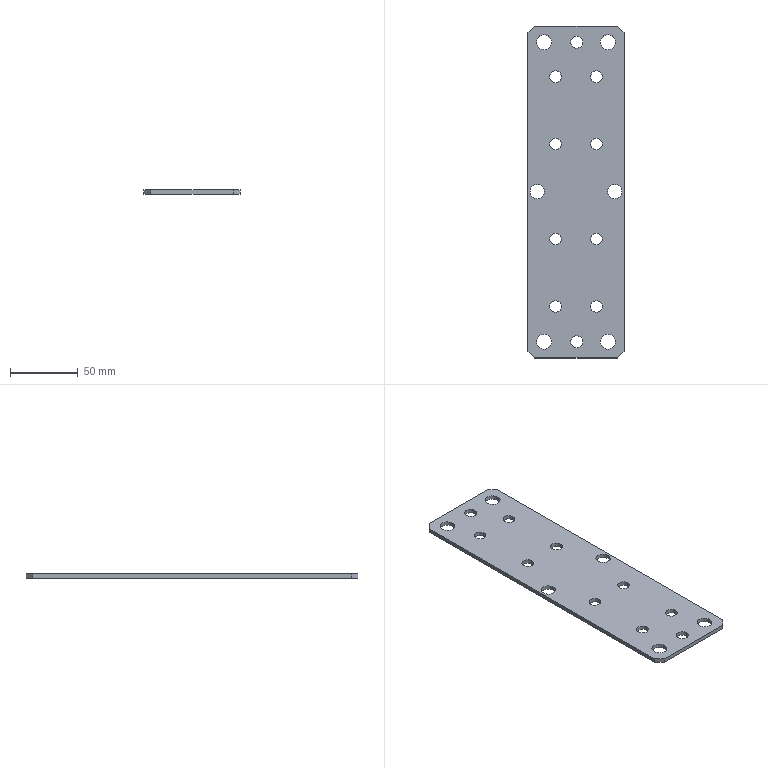Part | STEP file | 1_id266_x_t | 1 solid | 26 faces | box 70.8 x 244.8 x 3 mm | volume 48416 mm3 | cylinder 16 | plane 10 | commonest cylinder face diameters 8.6 x8 11 x4 8.938 x2 10.524 x2